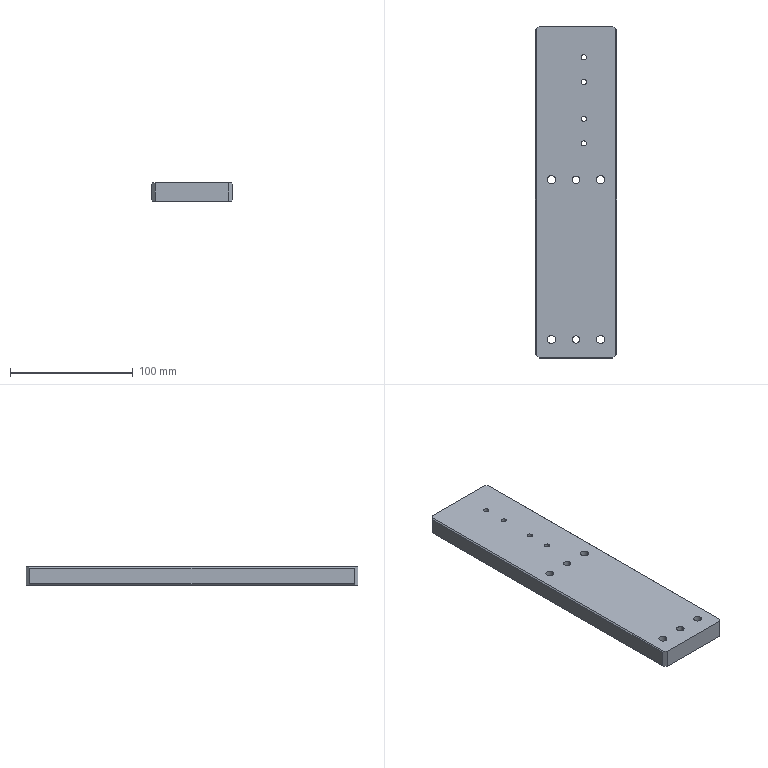Part | SolidWorks | features Chamfer 2, HoleWzd 2, ICE 2, Extrusion 1, MoveFace 1 | 1 solid | 52 faces | box 66 x 270 x 15 mm | volume 261133 mm3 | cylinder 32 | plane 20 | commonest cylinder face diameters 4.2 x8 6.6 x8 11 x8 6 x4 7 x4